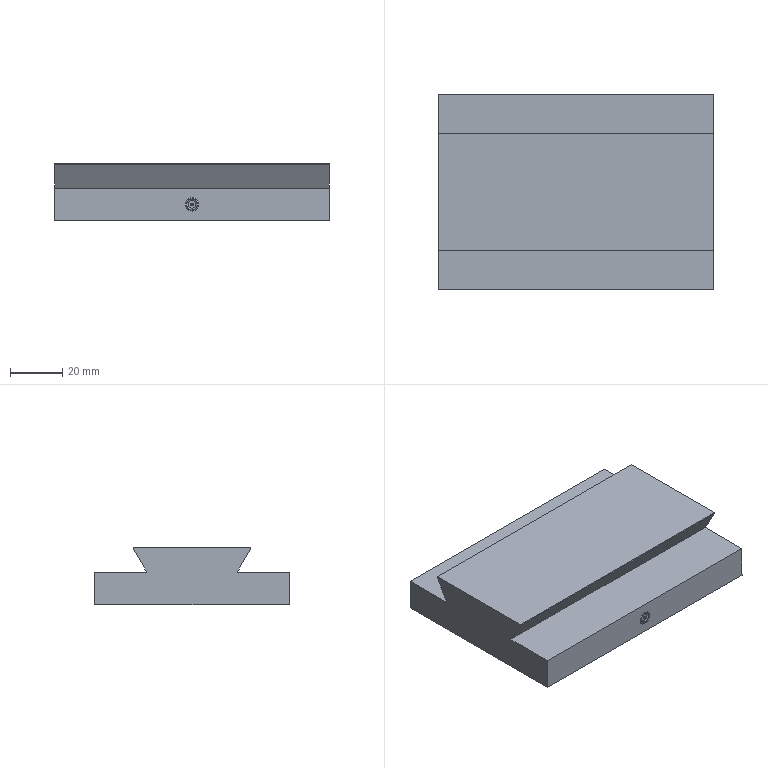Part | SolidWorks | features BaseBody 1 | 1 solid | 86 faces | box 105 x 74.5 x 22 mm | volume 135687 mm3 | cylinder 38 | cone 24 | plane 22 | torus 2 | commonest cylinder face diameters 4.134 x20 10 x12 1 x2 5 x2 5.1 x2